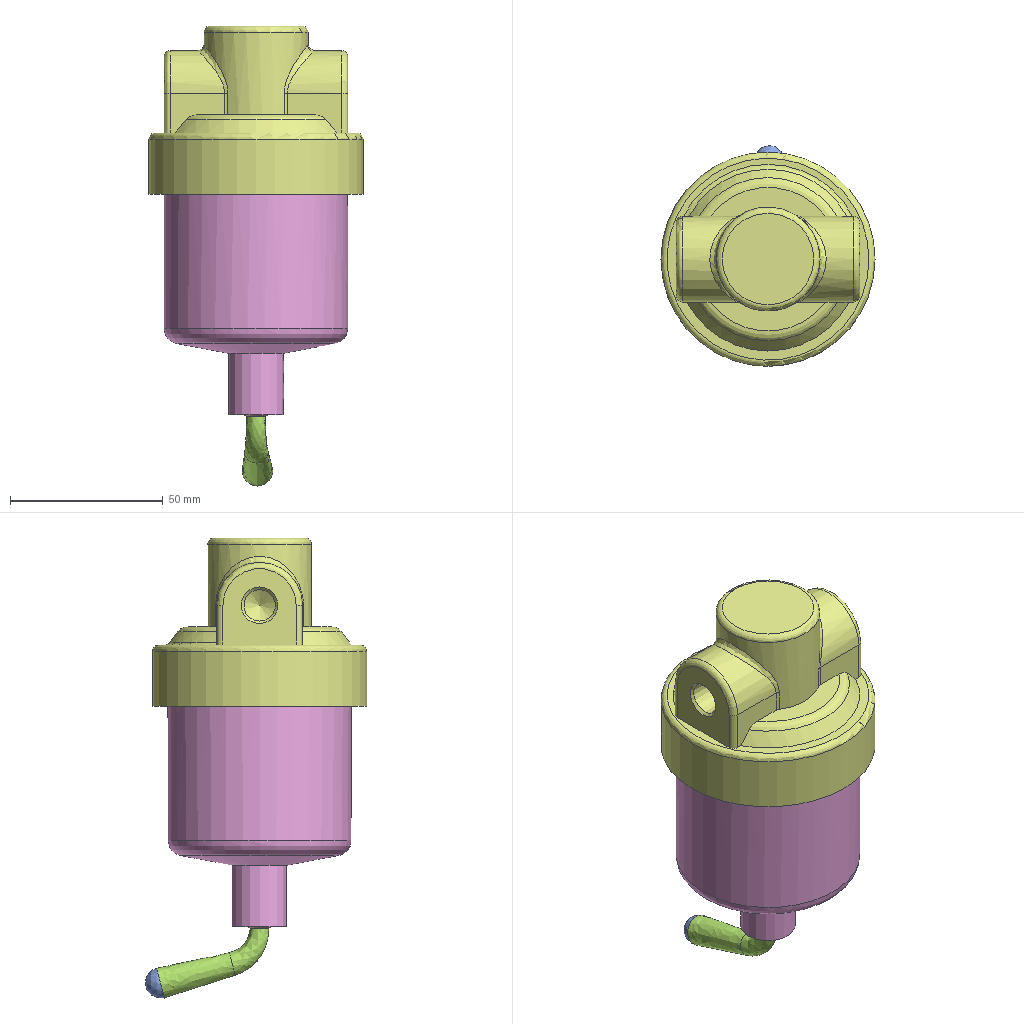Assembly | NX | 9 different items | 9 placed | box 70 x 72 x 150 mm
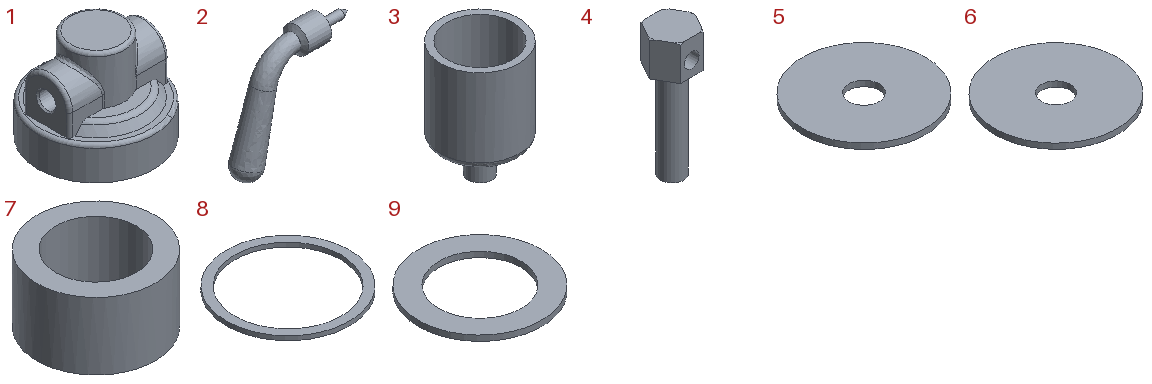Parts list (item | quantity | size | volume | features):
1 | x1 | 70 x 70 x 55 mm | 79994 mm3 | features CYLINDER 5, HOLE PACKAGE 5, SIMPLE HOLE 5, SYMBOLIC_THREAD 4, BLEND 3, DATUM_CSYS 2, BLOCK 1, SKETCH 1, SWP104 1
2 | x1 | 43.874 x 10 x 42.344 mm | 3412 mm3 | features SKETCH 4, DATUM_CSYS 3, DATUM_ON_PATH 2, SKIN 1, SPHERE 1, SWP104 1
3 | x1 | 60 x 60 x 88 mm | 68833 mm3 | features CYLINDER 3, BLEND 2, DATUM_CSYS 2, HOLE PACKAGE 2, SIMPLE HOLE 2, SYMBOLIC_THREAD 2, SKETCH 1, SWP104 1
4 | x1 | 18.475 x 16 x 52 mm | 4103 mm3 | features DATUM_CSYS 3, EXTRUDE 3, SKETCH 2, CHAMFER 1, CYLINDER 1, HOLE PACKAGE 1, SIMPLE HOLE 1, SYMBOLIC_THREAD 1
5 | x1 | 44 x 44 x 2 mm | 2851 mm3 | features CYLINDER 1, DATUM_CSYS 1, HOLE PACKAGE 1, SIMPLE HOLE 1
6 | x1 | 46 x 46 x 2 mm | 3134 mm3 | features CYLINDER 1, DATUM_CSYS 1, HOLE PACKAGE 1, SIMPLE HOLE 1
7 | x1 | 44.01 x 44.01 x 24.99 mm | 20351 mm3 | features CYLINDER 1, DATUM_CSYS 1, HOLE PACKAGE 1, SIMPLE HOLE 1
8 | x1 | 58 x 58 x 2 mm | 1357 mm3 | features CYLINDER 1, DATUM_CSYS 1, HOLE PACKAGE 1, SIMPLE HOLE 1
9 | x1 | 45 x 45 x 2 mm | 1767 mm3 | features CYLINDER 1, DATUM_CSYS 1, HOLE PACKAGE 1, SIMPLE HOLE 1
Mates (type | each side: item.copy, entity, surface, feature):
Touch | 8.1 face cylinder Ø50 Hole(2) | 1.1 face cylinder M10 x 1.5 Threaded Hole(17)
Touch | 8.1 face plane Cylinder(1) | 1.1 face plane Cylinder(11)
Touch | 9.1 face cylinder Ø30 Hole(2) | 1.1 face cylinder M10 x 1.5 Threaded Hole(17)
Touch | 9.1 face plane Cylinder(1) | 1.1 face plane Ø46 Hole(16)
Touch | 7.1 face cylinder Ø30 Hole(2) | 1.1 face cylinder M10 x 1.5 Threaded Hole(17)
Touch | 7.1 face plane Cylinder(1) | 1.1 face plane Ø46 Hole(16)
Touch | 6.1 face cylinder Ø11 Hole(2) | 7.1 face cylinder Ø30 Hole(2)
Touch | 6.1 face plane Cylinder(1) | 7.1 face plane Cylinder(1)
Touch | 5.1 face cylinder Ø11 Hole(2) | 6.1 face cylinder Ø11 Hole(2)
Touch | 5.1 face plane Cylinder(1) | 6.1 edge
Touch | 4.1 face cylinder Cylinder(5) | 7.1 face cylinder Cylinder(1)
Touch | 4.1 face plane Extrude(2) | 5.1 face plane Cylinder(1)
Touch | 3.1 face cylinder Revolve(2) | 7.1 face cylinder Cylinder(1)
Touch | 3.1 face plane Revolve(2) | 1.1 face plane Cylinder(11)
Fix | 3.1 component
Touch | 2.1 face cylinder Revolve(2) | 3.1 face cylinder M10 x 1.5 Threaded Hole(3)